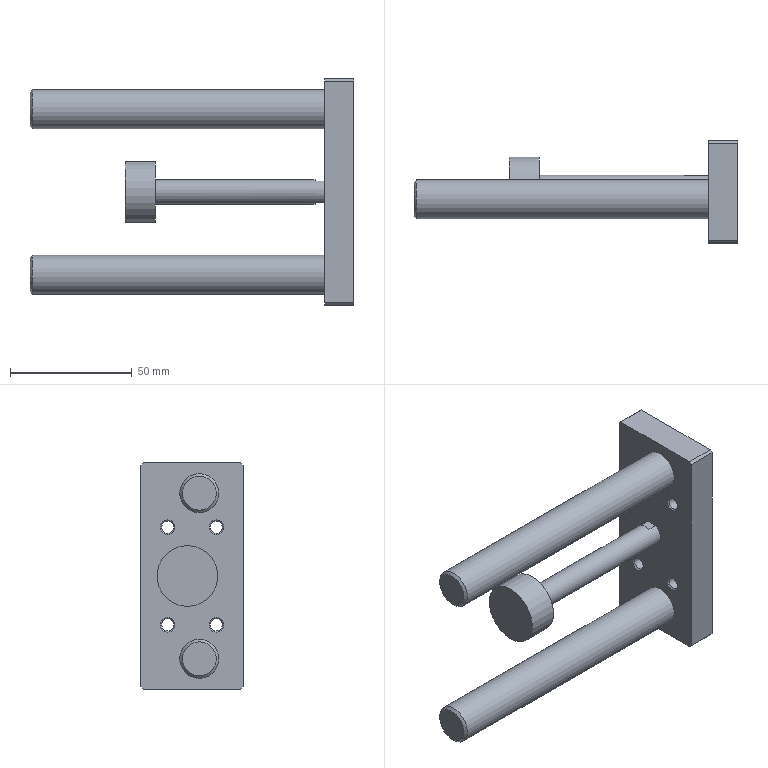Part | NX | features BREP 1 | 1 solid | 102 faces | box 133 x 42 x 93 mm | volume 105348 mm3 | cylinder 54 | plane 31 | cone 14 | torus 3 | commonest cylinder face diameters 1.12 x18 1.96 x18 4.917 x4 9 x4 10 x4 11 x3